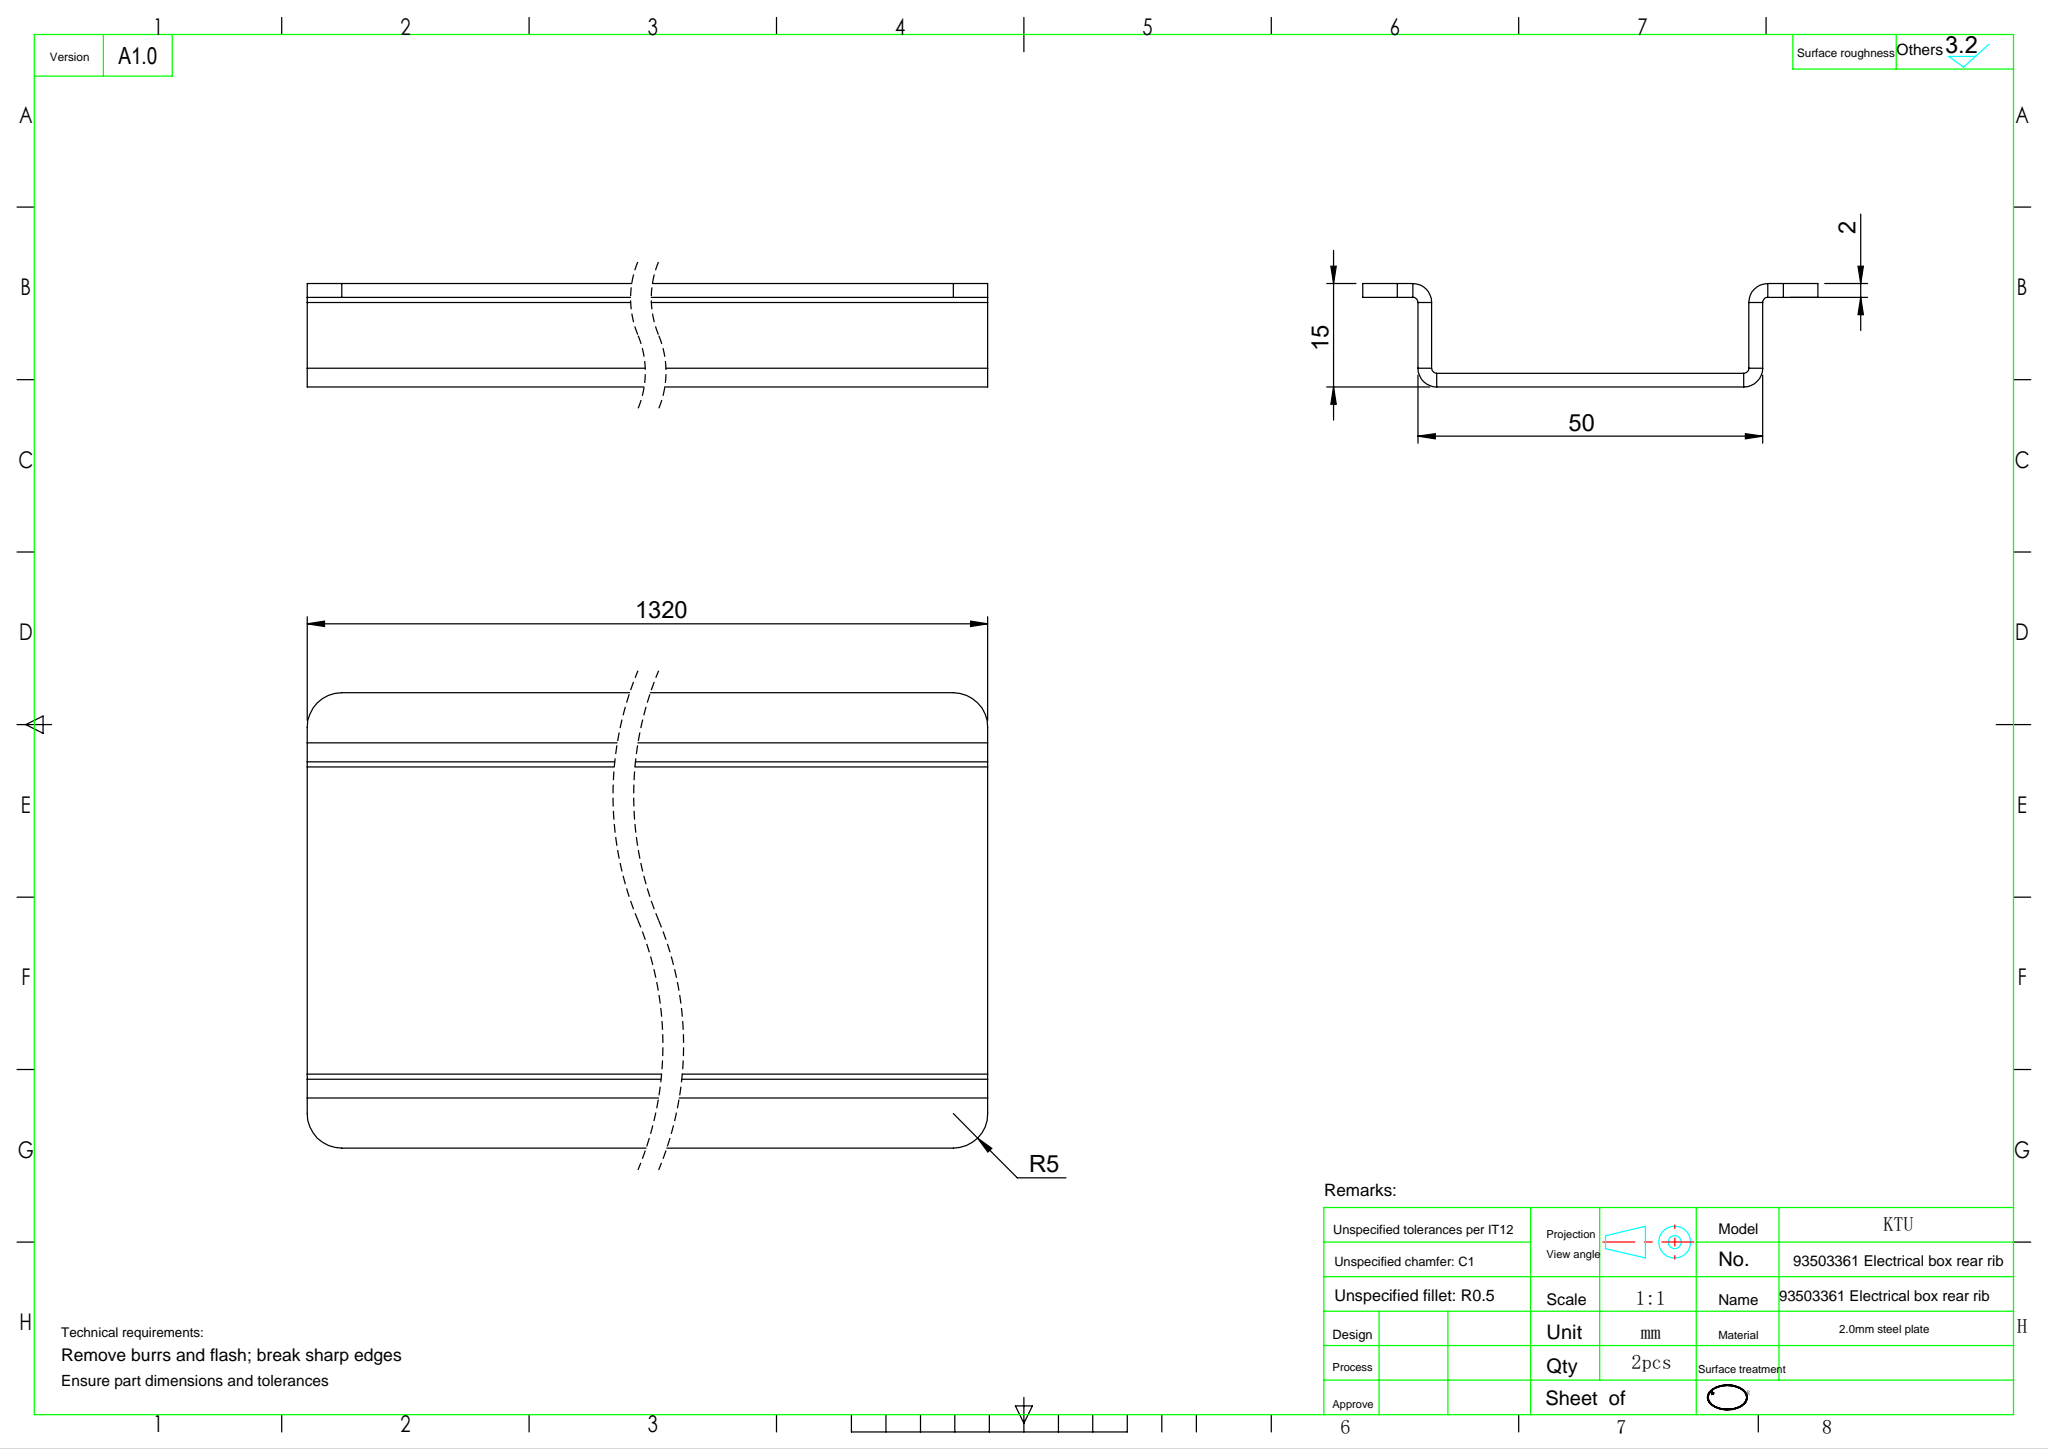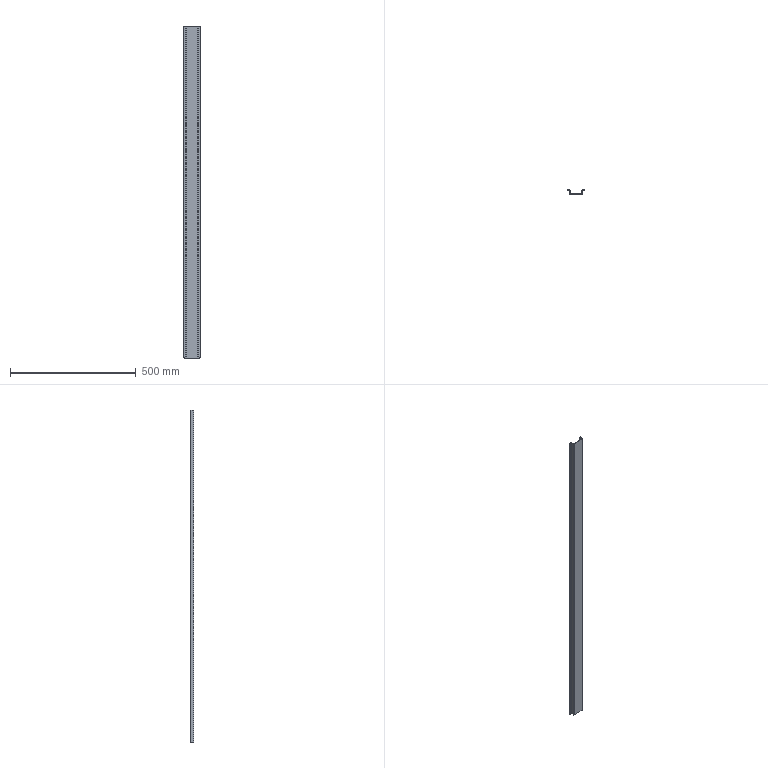Part | SolidWorks | features EdgeFlange 2, Fillet 1, FlatPattern 1, SMBaseFlange 1, SheetMetal 1 | 1 solid | 42 faces | box 66 x 15 x 1320 mm | volume 234966 mm3 | plane 30 | cylinder 12 | commonest cylinder face diameters 1.473 x4 5.473 x4 10 x4